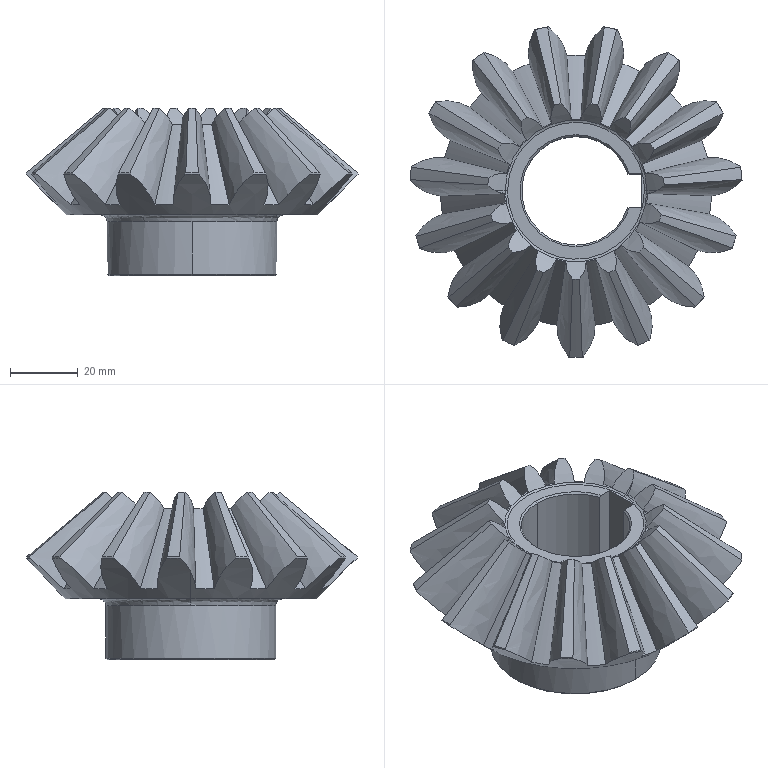Part | SolidWorks | features BaseBody 1 | 1 solid | 103 faces | box 97.808 x 97.316 x 49.456 mm | volume 114604 mm3 | cone 42 | spline 34 | cylinder 21 | plane 6 | commonest cylinder face diameters 98 x16 32 x3 50 x2